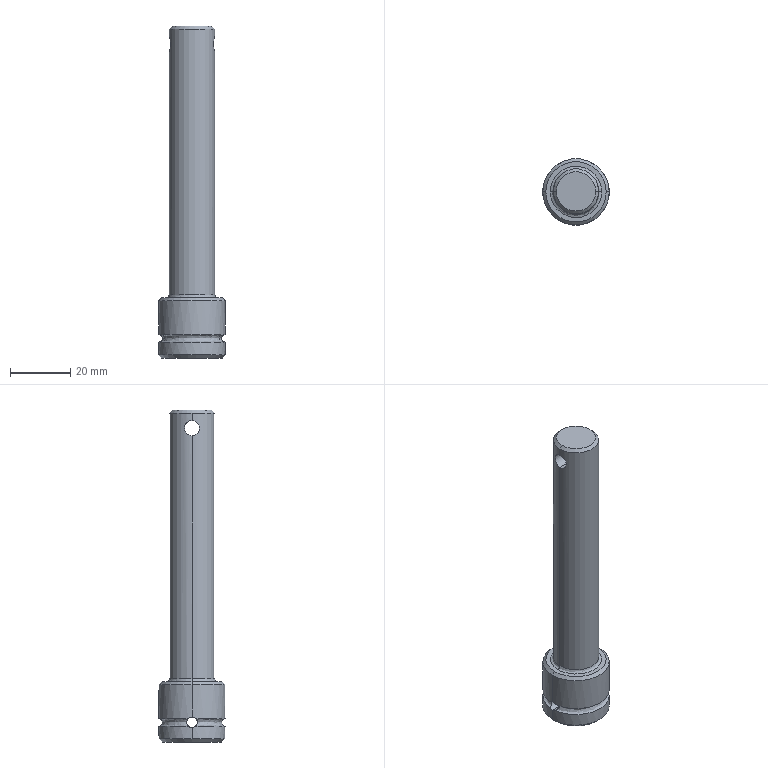Part | STEP file | fBY02F02M-00-15A | 1 solid | 34 faces | box 22 x 22 x 110 mm | volume 21708 mm3 | cylinder 16 | plane 8 | cone 6 | spline 4 | commonest cylinder face diameters 1 x4 3.5 x4 22 x4 5 x2 15 x2